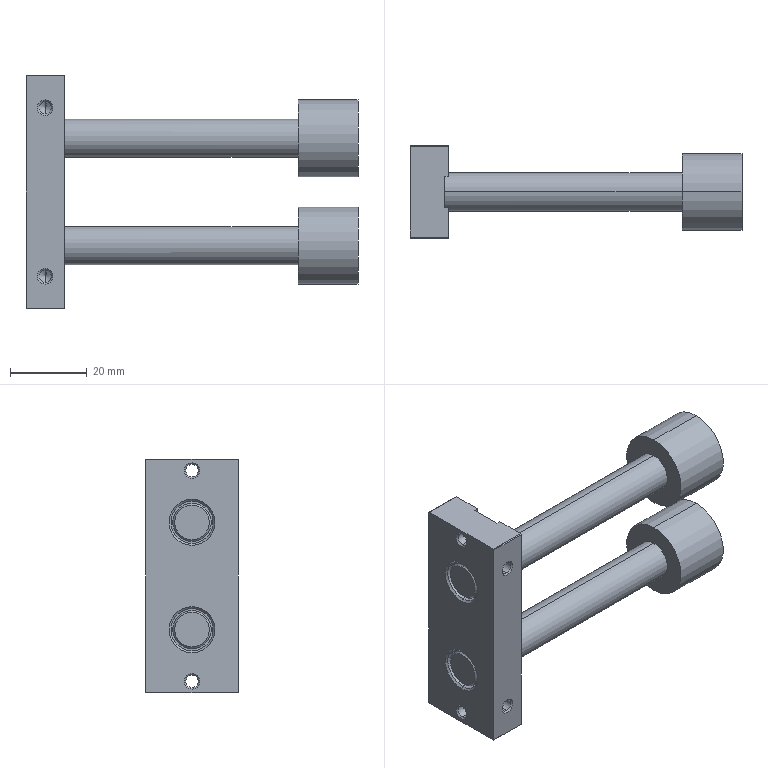Part | SolidWorks | features BaseBody 1 | 1 solid | 88 faces | box 86.6 x 24 x 61 mm | volume 33075 mm3 | cone 32 | cylinder 28 | plane 28 | commonest cylinder face diameters 3.242 x12 10 x8 11 x4 20 x4